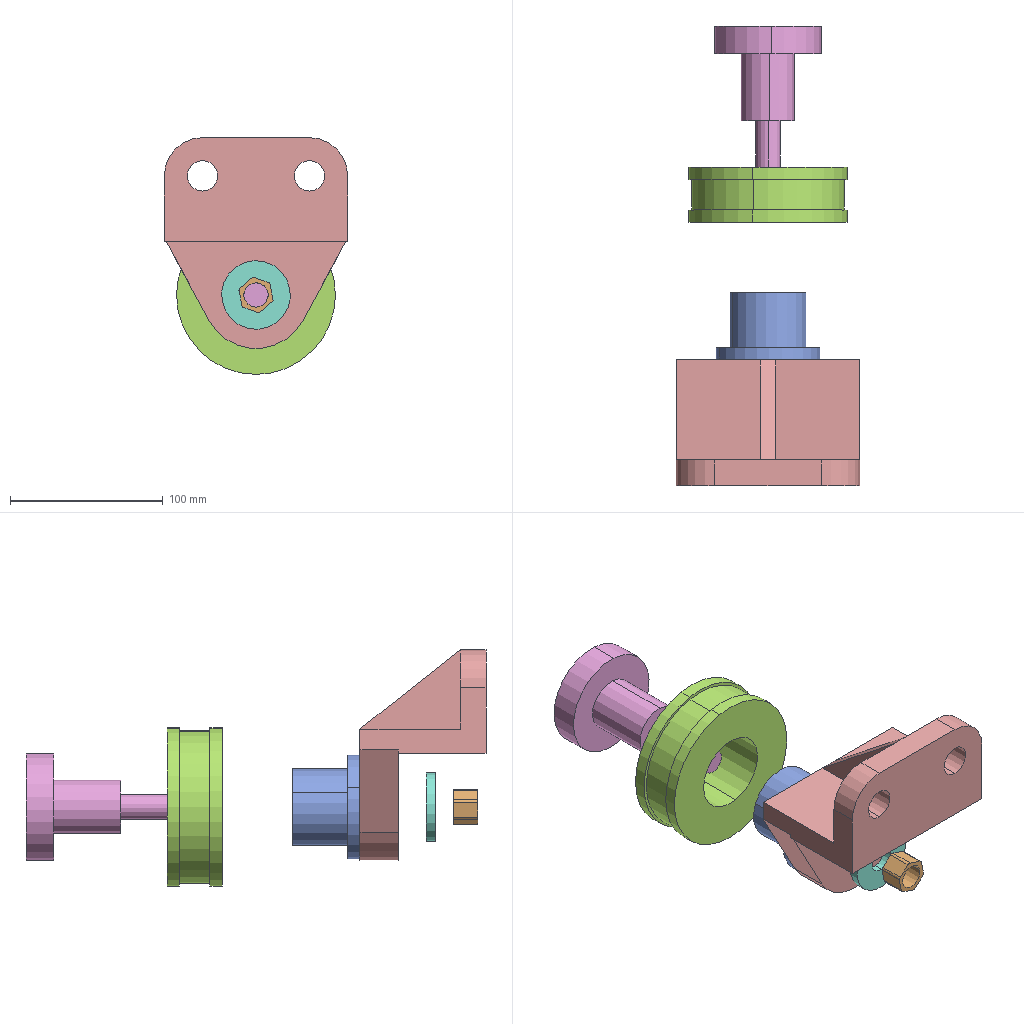Assembly | SolidWorks | 6 different items | 6 placed | box 120 x 301 x 155 mm
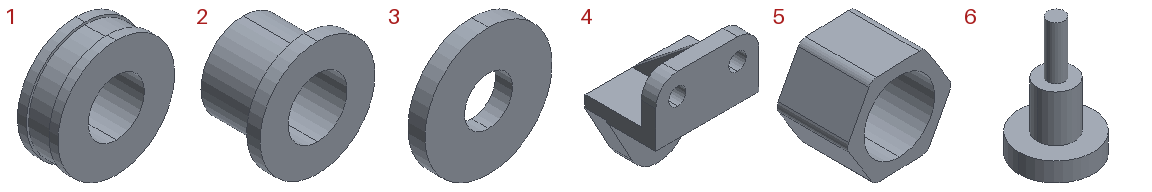Parts list (item | quantity | size | volume | features):
1 | x1 | 104 x 36 x 104 mm | 222312 mm3 | features ICE 3, Extrusion 1
2 | x1 | 68 x 44 x 68 mm | 57406 mm3 | features ICE 2, Extrusion 1
3 | x1 | 45 x 6 x 45 mm | 8181 mm3 | features Extrusion 1
4 | x1 | 120 x 82.471 x 138 mm | 396797 mm3 | features ICE 5, Extrusion 1
5 | x1 | 23.37 x 16 x 21.11 mm | 2748 mm3 | features Fillet 2, Extrusion 1
6 | x1 | 70 x 70 x 112 mm | 121658 mm3 | features Revolution 1
Mates (type | each side: item.copy, entity, surface, feature):
Coincident | 4.1 face plane Boss-Extrude1 | 2.1 face plane Boss-Extrude1
Concentric | 4.1 edge | 2.1 edge
Concentric | 2.1 face cylinder Boss-Extrude2 | 1.1 face cylinder Cut-Extrude1
Concentric | 4.1 face cylinder Cut-Extrude4 | 6.1 face cylinder Revolve1
Concentric | 6.1 face cylinder Revolve1 | 3.1 face cylinder Boss-Extrude1
Concentric | 6.1 face cylinder Revolve1 | 5.1 face cylinder Boss-Extrude1